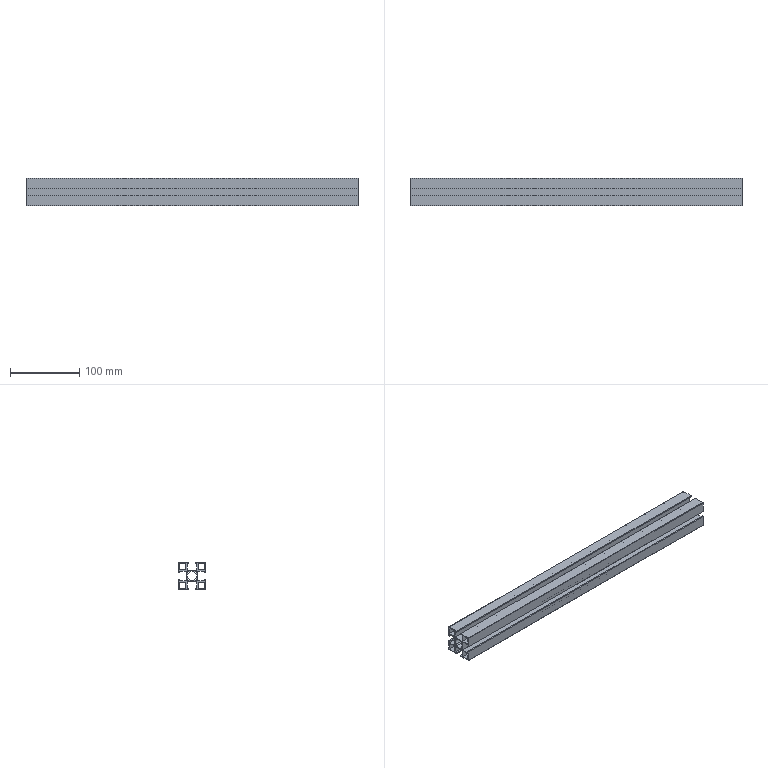Part | 1 solid | 77 faces | box 480 x 40 x 40 mm | volume 190267 mm3 | plane 62 | cylinder 15 | commonest cylinder face diameters 2.2 x6 14 x5 1 x4